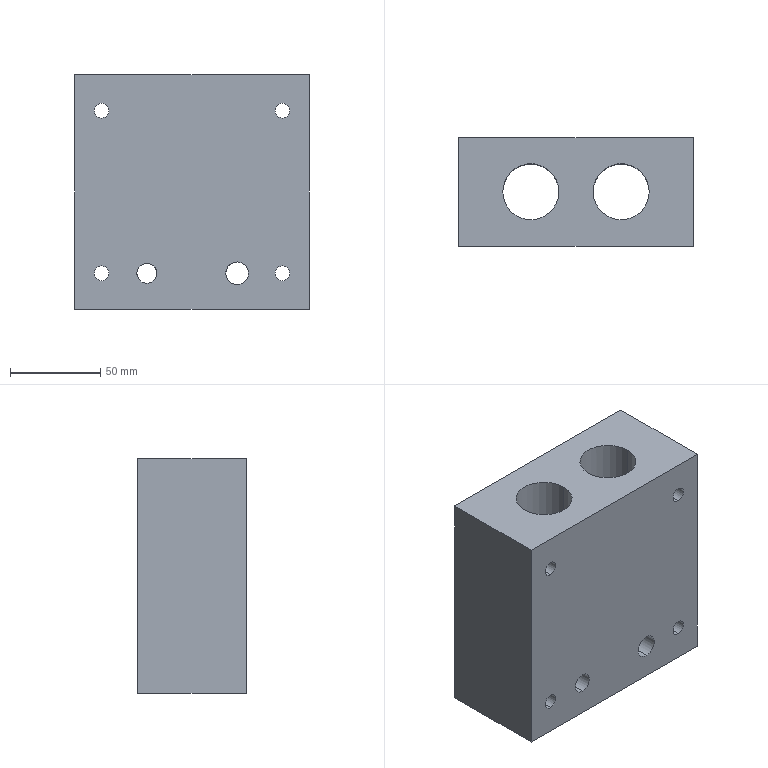Part | SolidWorks | features ICE 4, Extrusion 1 | 1 solid | 38 faces | box 130 x 60 x 130 mm | volume 778768 mm3 | cylinder 28 | plane 10 | commonest cylinder face diameters 8.2 x8 15 x8 11 x4 12.589 x4 31 x4